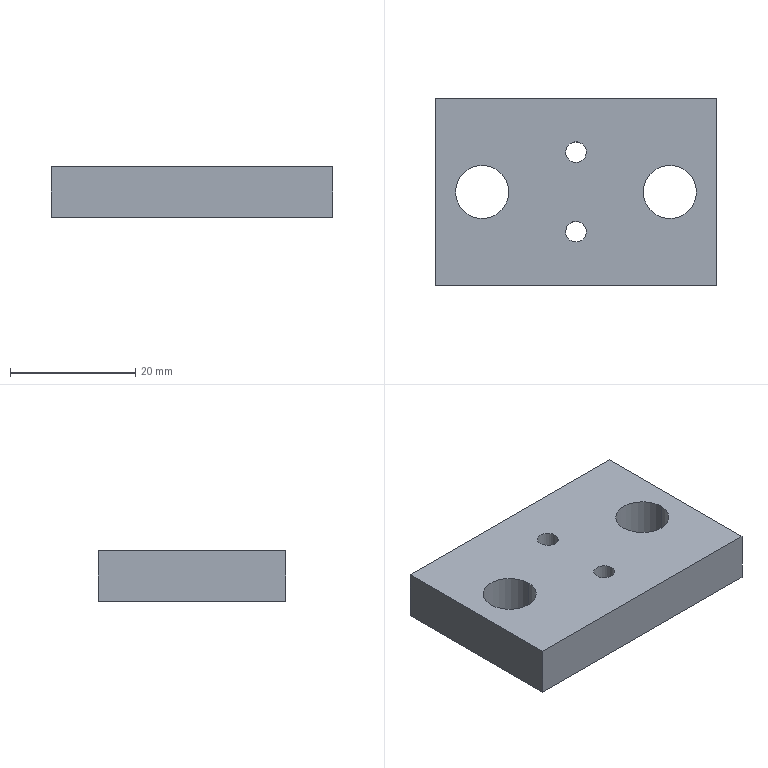Part | STEP file | 20308 | 1 solid | 14 faces | box 45 x 30 x 8 mm | volume 9755 mm3 | cylinder 8 | plane 6 | commonest cylinder face diameters 3.3 x4 8.5 x4
STEP:
#1=CARTESIAN_POINT('',(-1.448,7.141,0.));
#2=VERTEX_POINT('',#1);
#3=CARTESIAN_POINT('',(-1.448,7.141,8.));
#4=VERTEX_POINT('',#3);
#5=CARTESIAN_POINT('',(-1.448,7.141,-1.845));
#6=DIRECTION('',(0.,0.,-1.));
#7=VECTOR('',#6,1.);
#8=LINE('',#5,#7);
#9=EDGE_CURVE('',#2,#4,#8,.F.);
#10=ORIENTED_EDGE('',*,*,#9,.F.);
#11=CARTESIAN_POINT('',(1.448,5.559,0.));
#12=VERTEX_POINT('',#11);
#13=CARTESIAN_POINT('',(0.,6.35,0.));
#14=DIRECTION('',(0.,0.,-1.));
#15=AXIS2_PLACEMENT_3D('',#13,#14,$);
#16=CIRCLE('',#15,1.65);
#17=EDGE_CURVE('',#12,#2,#16,.F.);
#18=ORIENTED_EDGE('',*,*,#17,.F.);
#19=CARTESIAN_POINT('',(1.448,5.559,8.));
#20=VERTEX_POINT('',#19);
#21=CARTESIAN_POINT('',(1.448,5.559,-1.845));
#22=DIRECTION('',(0.,0.,-1.));
#23=VECTOR('',#22,1.);
#24=LINE('',#21,#23);
#25=EDGE_CURVE('',#12,#20,#24,.F.);
#26=ORIENTED_EDGE('',*,*,#25,.T.);
#27=CARTESIAN_POINT('',(0.,6.35,8.));
#28=DIRECTION('',(0.,0.,-1.));
#29=AXIS2_PLACEMENT_3D('',#27,#28,$);
#30=CIRCLE('',#29,1.65);
#31=EDGE_CURVE('',#20,#4,#30,.F.);
#32=ORIENTED_EDGE('',*,*,#31,.T.);
#33=EDGE_LOOP('',(#10,#18,#26,#32));
#34=FACE_OUTER_BOUND('',#33,.T.);
#35=CARTESIAN_POINT('',(0.,6.35,7.9));
#36=DIRECTION('',(0.,0.,-1.));
#37=DIRECTION('',(0.8776,-0.4794,0.));
#38=AXIS2_PLACEMENT_3D('',#35,#36,#37);
#39=CYLINDRICAL_SURFACE('',#38,1.65);
#40=ADVANCED_FACE('',(#34),#39,.F.);
#41=ORIENTED_EDGE('',*,*,#25,.F.);
#42=CARTESIAN_POINT('',(0.,6.35,0.));
#43=DIRECTION('',(0.,0.,-1.));
#44=AXIS2_PLACEMENT_3D('',#42,#43,$);
#45=CIRCLE('',#44,1.65);
#46=EDGE_CURVE('',#2,#12,#45,.F.);
#47=ORIENTED_EDGE('',*,*,#46,.F.);
#48=ORIENTED_EDGE('',*,*,#9,.T.);
#49=CARTESIAN_POINT('',(0.,6.35,8.));
#50=DIRECTION('',(0.,0.,-1.));
#51=AXIS2_PLACEMENT_3D('',#49,#50,$);
#52=CIRCLE('',#51,1.65);
#53=EDGE_CURVE('',#4,#20,#52,.F.);
#54=ORIENTED_EDGE('',*,*,#53,.T.);
#55=EDGE_LOOP('',(#41,#47,#48,#54));
#56=FACE_OUTER_BOUND('',#55,.T.);
#57=ADVANCED_FACE('',(#56),#39,.F.);
#58=CARTESIAN_POINT('',(22.5,15.,0.));
#59=VERTEX_POINT('',#58);
#60=CARTESIAN_POINT('',(22.5,15.,8.));
#61=VERTEX_POINT('',#60);
#62=CARTESIAN_POINT('',(22.5,15.,4.));
#63=DIRECTION('',(0.,0.,1.));
#64=VECTOR('',#63,1.);
#65=LINE('',#62,#64);
#66=EDGE_CURVE('',#59,#61,#65,.T.);
#67=ORIENTED_EDGE('',*,*,#66,.F.);
#68=CARTESIAN_POINT('',(-22.5,15.,0.));
#69=VERTEX_POINT('',#68);
#70=CARTESIAN_POINT('',(0.,15.,0.));
#71=DIRECTION('',(1.,0.,0.));
#72=VECTOR('',#71,1.);
#73=LINE('',#70,#72);
#74=EDGE_CURVE('',#59,#69,#73,.F.);
#75=ORIENTED_EDGE('',*,*,#74,.T.);
#76=CARTESIAN_POINT('',(-22.5,15.,8.));
#77=VERTEX_POINT('',#76);
#78=CARTESIAN_POINT('',(-22.5,15.,4.));
#79=DIRECTION('',(0.,0.,1.));
#80=VECTOR('',#79,1.);
#81=LINE('',#78,#80);
#82=EDGE_CURVE('',#69,#77,#81,.T.);
#83=ORIENTED_EDGE('',*,*,#82,.T.);
#84=CARTESIAN_POINT('',(0.,15.,8.));
#85=DIRECTION('',(1.,0.,0.));
#86=VECTOR('',#85,1.);
#87=LINE('',#84,#86);
#88=EDGE_CURVE('',#61,#77,#87,.F.);
#89=ORIENTED_EDGE('',*,*,#88,.F.);
#90=EDGE_LOOP('',(#67,#75,#83,#89));
#91=FACE_OUTER_BOUND('',#90,.T.);
#92=CARTESIAN_POINT('',(-22.5,15.,0.));
#93=DIRECTION('',(0.,-1.,0.));
#94=DIRECTION('',(1.,0.,0.));
#95=AXIS2_PLACEMENT_3D('',#92,#93,#94);
#96=PLANE('',#95);
#97=ADVANCED_FACE('',(#91),#96,.F.);
#98=ORIENTED_EDGE('',*,*,#82,.F.);
#99=CARTESIAN_POINT('',(-22.5,-15.,0.));
#100=VERTEX_POINT('',#99);
#101=CARTESIAN_POINT('',(-22.5,0.,0.));
#102=DIRECTION('',(0.,1.,0.));
#103=VECTOR('',#102,1.);
#104=LINE('',#101,#103);
#105=EDGE_CURVE('',#69,#100,#104,.F.);
#106=ORIENTED_EDGE('',*,*,#105,.T.);
#107=CARTESIAN_POINT('',(-22.5,-15.,8.));
#108=VERTEX_POINT('',#107);
#109=CARTESIAN_POINT('',(-22.5,-15.,4.));
#110=DIRECTION('',(0.,0.,1.));
#111=VECTOR('',#110,1.);
#112=LINE('',#109,#111);
#113=EDGE_CURVE('',#100,#108,#112,.T.);
#114=ORIENTED_EDGE('',*,*,#113,.T.);
#115=CARTESIAN_POINT('',(-22.5,0.,8.));
#116=DIRECTION('',(0.,1.,0.));
#117=VECTOR('',#116,1.);
#118=LINE('',#115,#117);
#119=EDGE_CURVE('',#77,#108,#118,.F.);
#120=ORIENTED_EDGE('',*,*,#119,.F.);
#121=EDGE_LOOP('',(#98,#106,#114,#120));
#122=FACE_OUTER_BOUND('',#121,.T.);
#123=CARTESIAN_POINT('',(-22.5,-15.,0.));
#124=DIRECTION('',(1.,0.,0.));
#125=DIRECTION('',(0.,1.,0.));
#126=AXIS2_PLACEMENT_3D('',#123,#124,#125);
#127=PLANE('',#126);
#128=ADVANCED_FACE('',(#122),#127,.F.);
#129=ORIENTED_EDGE('',*,*,#113,.F.);
#130=CARTESIAN_POINT('',(22.5,-15.,0.));
#131=VERTEX_POINT('',#130);
#132=CARTESIAN_POINT('',(0.,-15.,0.));
#133=DIRECTION('',(-1.,0.,0.));
#134=VECTOR('',#133,1.);
#135=LINE('',#132,#134);
#136=EDGE_CURVE('',#100,#131,#135,.F.);
#137=ORIENTED_EDGE('',*,*,#136,.T.);
#138=CARTESIAN_POINT('',(22.5,-15.,8.));
#139=VERTEX_POINT('',#138);
#140=CARTESIAN_POINT('',(22.5,-15.,4.));
#141=DIRECTION('',(0.,0.,1.));
#142=VECTOR('',#141,1.);
#143=LINE('',#140,#142);
#144=EDGE_CURVE('',#131,#139,#143,.T.);
#145=ORIENTED_EDGE('',*,*,#144,.T.);
#146=CARTESIAN_POINT('',(0.,-15.,8.));
#147=DIRECTION('',(-1.,0.,0.));
#148=VECTOR('',#147,1.);
#149=LINE('',#146,#148);
#150=EDGE_CURVE('',#108,#139,#149,.F.);
#151=ORIENTED_EDGE('',*,*,#150,.F.);
#152=EDGE_LOOP('',(#129,#137,#145,#151));
#153=FACE_OUTER_BOUND('',#152,.T.);
#154=CARTESIAN_POINT('',(22.5,-15.,0.));
#155=DIRECTION('',(0.,1.,0.));
#156=DIRECTION('',(-1.,0.,0.));
#157=AXIS2_PLACEMENT_3D('',#154,#155,#156);
#158=PLANE('',#157);
#159=ADVANCED_FACE('',(#153),#158,.F.);
#160=ORIENTED_EDGE('',*,*,#144,.F.);
#161=CARTESIAN_POINT('',(22.5,0.,0.));
#162=DIRECTION('',(0.,-1.,0.));
#163=VECTOR('',#162,1.);
#164=LINE('',#161,#163);
#165=EDGE_CURVE('',#131,#59,#164,.F.);
#166=ORIENTED_EDGE('',*,*,#165,.T.);
#167=ORIENTED_EDGE('',*,*,#66,.T.);
#168=CARTESIAN_POINT('',(22.5,0.,8.));
#169=DIRECTION('',(0.,-1.,0.));
#170=VECTOR('',#169,1.);
#171=LINE('',#168,#170);
#172=EDGE_CURVE('',#139,#61,#171,.F.);
#173=ORIENTED_EDGE('',*,*,#172,.F.);
#174=EDGE_LOOP('',(#160,#166,#167,#173));
#175=FACE_OUTER_BOUND('',#174,.T.);
#176=CARTESIAN_POINT('',(22.5,15.,0.));
#177=DIRECTION('',(-1.,0.,0.));
#178=DIRECTION('',(0.,-1.,0.));
#179=AXIS2_PLACEMENT_3D('',#176,#177,#178);
#180=PLANE('',#179);
#181=ADVANCED_FACE('',(#175),#180,.F.);
#182=CARTESIAN_POINT('',(10.75,0.,8.));
#183=VERTEX_POINT('',#182);
#184=CARTESIAN_POINT('',(19.25,0.,8.));
#185=VERTEX_POINT('',#184);
#186=CARTESIAN_POINT('',(15.,0.,8.));
#187=DIRECTION('',(0.,0.,1.));
#188=AXIS2_PLACEMENT_3D('',#186,#187,$);
#189=CIRCLE('',#188,4.25);
#190=EDGE_CURVE('',#183,#185,#189,.T.);
#191=ORIENTED_EDGE('',*,*,#190,.T.);
#192=CARTESIAN_POINT('',(19.25,0.,0.));
#193=VERTEX_POINT('',#192);
#194=CARTESIAN_POINT('',(19.25,0.,4.));
#195=DIRECTION('',(0.,0.,1.));
#196=VECTOR('',#195,1.);
#197=LINE('',#194,#196);
#198=EDGE_CURVE('',#193,#185,#197,.T.);
#199=ORIENTED_EDGE('',*,*,#198,.F.);
#200=CARTESIAN_POINT('',(10.75,0.,0.));
#201=VERTEX_POINT('',#200);
#202=CARTESIAN_POINT('',(15.,0.,0.));
#203=DIRECTION('',(0.,0.,1.));
#204=AXIS2_PLACEMENT_3D('',#202,#203,$);
#205=CIRCLE('',#204,4.25);
#206=EDGE_CURVE('',#201,#193,#205,.T.);
#207=ORIENTED_EDGE('',*,*,#206,.F.);
#208=CARTESIAN_POINT('',(10.75,0.,4.));
#209=DIRECTION('',(0.,0.,1.));
#210=VECTOR('',#209,1.);
#211=LINE('',#208,#210);
#212=EDGE_CURVE('',#201,#183,#211,.T.);
#213=ORIENTED_EDGE('',*,*,#212,.T.);
#214=EDGE_LOOP('',(#191,#199,#207,#213));
#215=FACE_OUTER_BOUND('',#214,.T.);
#216=CARTESIAN_POINT('',(15.,0.,4.));
#217=DIRECTION('',(0.,0.,1.));
#218=DIRECTION('',(-1.,0.,0.));
#219=AXIS2_PLACEMENT_3D('',#216,#217,#218);
#220=CYLINDRICAL_SURFACE('',#219,4.25);
#221=ADVANCED_FACE('',(#215),#220,.F.);
#222=CARTESIAN_POINT('',(15.,0.,8.));
#223=DIRECTION('',(0.,0.,1.));
#224=AXIS2_PLACEMENT_3D('',#222,#223,$);
#225=CIRCLE('',#224,4.25);
#226=EDGE_CURVE('',#185,#183,#225,.T.);
#227=ORIENTED_EDGE('',*,*,#226,.T.);
#228=ORIENTED_EDGE('',*,*,#212,.F.);
#229=CARTESIAN_POINT('',(15.,0.,0.));
#230=DIRECTION('',(0.,0.,1.));
#231=AXIS2_PLACEMENT_3D('',#229,#230,$);
#232=CIRCLE('',#231,4.25);
#233=EDGE_CURVE('',#193,#201,#232,.T.);
#234=ORIENTED_EDGE('',*,*,#233,.F.);
#235=ORIENTED_EDGE('',*,*,#198,.T.);
#236=EDGE_LOOP('',(#227,#228,#234,#235));
#237=FACE_OUTER_BOUND('',#236,.T.);
#238=ADVANCED_FACE('',(#237),#220,.F.);
#239=CARTESIAN_POINT('',(-10.75,0.,8.));
#240=VERTEX_POINT('',#239);
#241=CARTESIAN_POINT('',(-19.25,0.,8.));
#242=VERTEX_POINT('',#241);
#243=CARTESIAN_POINT('',(-15.,0.,8.));
#244=DIRECTION('',(0.,0.,1.));
#245=AXIS2_PLACEMENT_3D('',#243,#244,$);
#246=CIRCLE('',#245,4.25);
#247=EDGE_CURVE('',#240,#242,#246,.T.);
#248=ORIENTED_EDGE('',*,*,#247,.T.);
#249=CARTESIAN_POINT('',(-19.25,0.,0.));
#250=VERTEX_POINT('',#249);
#251=CARTESIAN_POINT('',(-19.25,0.,4.));
#252=DIRECTION('',(0.,0.,1.));
#253=VECTOR('',#252,1.);
#254=LINE('',#251,#253);
#255=EDGE_CURVE('',#250,#242,#254,.T.);
#256=ORIENTED_EDGE('',*,*,#255,.F.);
#257=CARTESIAN_POINT('',(-10.75,0.,0.));
#258=VERTEX_POINT('',#257);
#259=CARTESIAN_POINT('',(-15.,0.,0.));
#260=DIRECTION('',(0.,0.,1.));
#261=AXIS2_PLACEMENT_3D('',#259,#260,$);
#262=CIRCLE('',#261,4.25);
#263=EDGE_CURVE('',#258,#250,#262,.T.);
#264=ORIENTED_EDGE('',*,*,#263,.F.);
#265=CARTESIAN_POINT('',(-10.75,0.,4.));
#266=DIRECTION('',(0.,0.,1.));
#267=VECTOR('',#266,1.);
#268=LINE('',#265,#267);
#269=EDGE_CURVE('',#258,#240,#268,.T.);
#270=ORIENTED_EDGE('',*,*,#269,.T.);
#271=EDGE_LOOP('',(#248,#256,#264,#270));
#272=FACE_OUTER_BOUND('',#271,.T.);
#273=CARTESIAN_POINT('',(-15.,0.,4.));
#274=DIRECTION('',(0.,0.,1.));
#275=DIRECTION('',(1.,0.,0.));
#276=AXIS2_PLACEMENT_3D('',#273,#274,#275);
#277=CYLINDRICAL_SURFACE('',#276,4.25);
#278=ADVANCED_FACE('',(#272),#277,.F.);
#279=CARTESIAN_POINT('',(-15.,0.,8.));
#280=DIRECTION('',(0.,0.,1.));
#281=AXIS2_PLACEMENT_3D('',#279,#280,$);
#282=CIRCLE('',#281,4.25);
#283=EDGE_CURVE('',#242,#240,#282,.T.);
#284=ORIENTED_EDGE('',*,*,#283,.T.);
#285=ORIENTED_EDGE('',*,*,#269,.F.);
#286=CARTESIAN_POINT('',(-15.,0.,0.));
#287=DIRECTION('',(0.,0.,1.));
#288=AXIS2_PLACEMENT_3D('',#286,#287,$);
#289=CIRCLE('',#288,4.25);
#290=EDGE_CURVE('',#250,#258,#289,.T.);
#291=ORIENTED_EDGE('',*,*,#290,.F.);
#292=ORIENTED_EDGE('',*,*,#255,.T.);
#293=EDGE_LOOP('',(#284,#285,#291,#292));
#294=FACE_OUTER_BOUND('',#293,.T.);
#295=ADVANCED_FACE('',(#294),#277,.F.);
#296=ORIENTED_EDGE('',*,*,#165,.F.);
#297=ORIENTED_EDGE('',*,*,#136,.F.);
#298=ORIENTED_EDGE('',*,*,#105,.F.);
#299=ORIENTED_EDGE('',*,*,#74,.F.);
#300=EDGE_LOOP('',(#296,#297,#298,#299));
#301=FACE_OUTER_BOUND('',#300,.T.);
#302=CARTESIAN_POINT('',(-1.448,-5.559,0.));
#303=VERTEX_POINT('',#302);
#304=CARTESIAN_POINT('',(1.448,-7.141,0.));
#305=VERTEX_POINT('',#304);
#306=CARTESIAN_POINT('',(0.,-6.35,0.));
#307=DIRECTION('',(0.,0.,1.));
#308=AXIS2_PLACEMENT_3D('',#306,#307,$);
#309=CIRCLE('',#308,1.65);
#310=EDGE_CURVE('',#303,#305,#309,.T.);
#311=ORIENTED_EDGE('',*,*,#310,.T.);
#312=CARTESIAN_POINT('',(0.,-6.35,0.));
#313=DIRECTION('',(0.,0.,1.));
#314=AXIS2_PLACEMENT_3D('',#312,#313,$);
#315=CIRCLE('',#314,1.65);
#316=EDGE_CURVE('',#305,#303,#315,.T.);
#317=ORIENTED_EDGE('',*,*,#316,.T.);
#318=EDGE_LOOP('',(#311,#317));
#319=FACE_BOUND('',#318,.T.);
#320=ORIENTED_EDGE('',*,*,#17,.T.);
#321=ORIENTED_EDGE('',*,*,#46,.T.);
#322=EDGE_LOOP('',(#320,#321));
#323=FACE_BOUND('',#322,.T.);
#324=ORIENTED_EDGE('',*,*,#263,.T.);
#325=ORIENTED_EDGE('',*,*,#290,.T.);
#326=EDGE_LOOP('',(#324,#325));
#327=FACE_BOUND('',#326,.T.);
#328=ORIENTED_EDGE('',*,*,#206,.T.);
#329=ORIENTED_EDGE('',*,*,#233,.T.);
#330=EDGE_LOOP('',(#328,#329));
#331=FACE_BOUND('',#330,.T.);
#332=CARTESIAN_POINT('',(0.,0.,0.));
#333=DIRECTION('',(0.,0.,1.));
#334=DIRECTION('',(1.,0.,0.));
#335=AXIS2_PLACEMENT_3D('',#332,#333,#334);
#336=PLANE('',#335);
#337=ADVANCED_FACE('',(#301,#319,#323,#327,#331),#336,.F.);
#338=ORIENTED_EDGE('',*,*,#88,.T.);
#339=ORIENTED_EDGE('',*,*,#119,.T.);
#340=ORIENTED_EDGE('',*,*,#150,.T.);
#341=ORIENTED_EDGE('',*,*,#172,.T.);
#342=EDGE_LOOP('',(#338,#339,#340,#341));
#343=FACE_OUTER_BOUND('',#342,.T.);
#344=CARTESIAN_POINT('',(1.448,-7.141,8.));
#345=VERTEX_POINT('',#344);
#346=CARTESIAN_POINT('',(-1.448,-5.559,8.));
#347=VERTEX_POINT('',#346);
#348=CARTESIAN_POINT('',(0.,-6.35,8.));
#349=DIRECTION('',(0.,0.,1.));
#350=AXIS2_PLACEMENT_3D('',#348,#349,$);
#351=CIRCLE('',#350,1.65);
#352=EDGE_CURVE('',#345,#347,#351,.T.);
#353=ORIENTED_EDGE('',*,*,#352,.F.);
#354=CARTESIAN_POINT('',(0.,-6.35,8.));
#355=DIRECTION('',(0.,0.,1.));
#356=AXIS2_PLACEMENT_3D('',#354,#355,$);
#357=CIRCLE('',#356,1.65);
#358=EDGE_CURVE('',#347,#345,#357,.T.);
#359=ORIENTED_EDGE('',*,*,#358,.F.);
#360=EDGE_LOOP('',(#353,#359));
#361=FACE_BOUND('',#360,.T.);
#362=ORIENTED_EDGE('',*,*,#53,.F.);
#363=ORIENTED_EDGE('',*,*,#31,.F.);
#364=EDGE_LOOP('',(#362,#363));
#365=FACE_BOUND('',#364,.T.);
#366=ORIENTED_EDGE('',*,*,#283,.F.);
#367=ORIENTED_EDGE('',*,*,#247,.F.);
#368=EDGE_LOOP('',(#366,#367));
#369=FACE_BOUND('',#368,.T.);
#370=ORIENTED_EDGE('',*,*,#226,.F.);
#371=ORIENTED_EDGE('',*,*,#190,.F.);
#372=EDGE_LOOP('',(#370,#371));
#373=FACE_BOUND('',#372,.T.);
#374=CARTESIAN_POINT('',(0.,0.,8.));
#375=DIRECTION('',(0.,0.,1.));
#376=DIRECTION('',(1.,0.,0.));
#377=AXIS2_PLACEMENT_3D('',#374,#375,#376);
#378=PLANE('',#377);
#379=ADVANCED_FACE('',(#343,#361,#365,#369,#373),#378,.T.);
#380=CARTESIAN_POINT('',(-1.448,-5.559,-1.845));
#381=DIRECTION('',(0.,0.,-1.));
#382=VECTOR('',#381,1.);
#383=LINE('',#380,#382);
#384=EDGE_CURVE('',#303,#347,#383,.F.);
#385=ORIENTED_EDGE('',*,*,#384,.F.);
#386=ORIENTED_EDGE('',*,*,#316,.F.);
#387=CARTESIAN_POINT('',(1.448,-7.141,-1.845));
#388=DIRECTION('',(0.,0.,-1.));
#389=VECTOR('',#388,1.);
#390=LINE('',#387,#389);
#391=EDGE_CURVE('',#305,#345,#390,.F.);
#392=ORIENTED_EDGE('',*,*,#391,.T.);
#393=ORIENTED_EDGE('',*,*,#352,.T.);
#394=EDGE_LOOP('',(#385,#386,#392,#393));
#395=FACE_OUTER_BOUND('',#394,.T.);
#396=CARTESIAN_POINT('',(0.,-6.35,7.9));
#397=DIRECTION('',(0.,0.,-1.));
#398=DIRECTION('',(0.8776,-0.4794,0.));
#399=AXIS2_PLACEMENT_3D('',#396,#397,#398);
#400=CYLINDRICAL_SURFACE('',#399,1.65);
#401=ADVANCED_FACE('',(#395),#400,.F.);
#402=ORIENTED_EDGE('',*,*,#391,.F.);
#403=ORIENTED_EDGE('',*,*,#310,.F.);
#404=ORIENTED_EDGE('',*,*,#384,.T.);
#405=ORIENTED_EDGE('',*,*,#358,.T.);
#406=EDGE_LOOP('',(#402,#403,#404,#405));
#407=FACE_OUTER_BOUND('',#406,.T.);
#408=ADVANCED_FACE('',(#407),#400,.F.);
#409=CLOSED_SHELL('',(#40,#57,#97,#128,#159,#181,#221,#238,#278,#295,#337,#379,#401,#408));
#410=MANIFOLD_SOLID_BREP('',#409);
#411=(LENGTH_UNIT()NAMED_UNIT(*)SI_UNIT(.MILLI.,.METRE.));
#412=UNCERTAINTY_MEASURE_WITH_UNIT(LENGTH_MEASURE(0.005),#411,'','');
#413=(NAMED_UNIT(*)PLANE_ANGLE_UNIT()SI_UNIT($,.RADIAN.));
#414=(NAMED_UNIT(*)SI_UNIT($,.STERADIAN.)SOLID_ANGLE_UNIT());
#415=(GEOMETRIC_REPRESENTATION_CONTEXT(3)GLOBAL_UNCERTAINTY_ASSIGNED_CONTEXT((#412))GLOBAL_UNIT_ASSIGNED_CONTEXT((#411,#413,#414))REPRESENTATION_CONTEXT('',''));
#416=ADVANCED_BREP_SHAPE_REPRESENTATION('',(#410),#415);